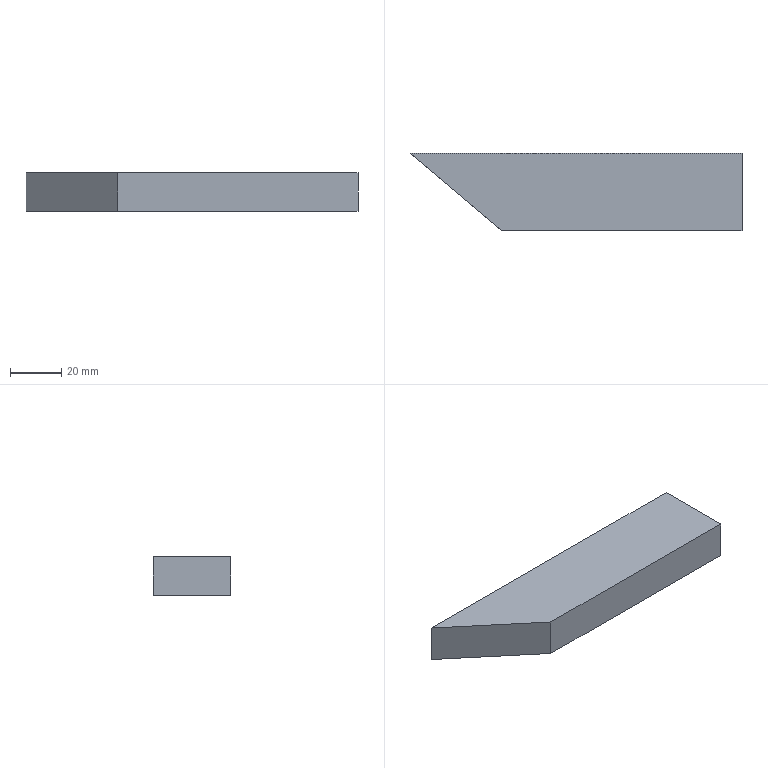Part | NX | features solid 2 | 1 solid | 6 faces | box 129.171 x 30 x 15 mm | volume 50083 mm3 | plane 6
STEP:
#1=CARTESIAN_POINT('',(-96.794,70.,-30.));
#2=VERTEX_POINT('',#1);
#3=CARTESIAN_POINT('',(-61.041,40.,-30.));
#4=VERTEX_POINT('',#3);
#5=CARTESIAN_POINT('',(-95.209,68.67,-30.));
#6=DIRECTION('',(0.766,-0.6428,0.));
#7=VECTOR('',#6,1000.);
#8=LINE('',#5,#7);
#9=EDGE_CURVE('',#2,#4,#8,.T.);
#10=ORIENTED_EDGE('',*,*,#9,.T.);
#11=CARTESIAN_POINT('',(-61.041,40.,-15.));
#12=VERTEX_POINT('',#11);
#13=CARTESIAN_POINT('',(-61.041,40.,-30.));
#14=DIRECTION('',(0.,0.,1.));
#15=VECTOR('',#14,1000.);
#16=LINE('',#13,#15);
#17=EDGE_CURVE('',#4,#12,#16,.T.);
#18=ORIENTED_EDGE('',*,*,#17,.T.);
#19=CARTESIAN_POINT('',(-96.794,70.,-15.));
#20=VERTEX_POINT('',#19);
#21=CARTESIAN_POINT('',(-62.071,40.864,-15.));
#22=DIRECTION('',(-0.766,0.6428,0.));
#23=VECTOR('',#22,1000.);
#24=LINE('',#21,#23);
#25=EDGE_CURVE('',#20,#12,#24,.F.);
#26=ORIENTED_EDGE('',*,*,#25,.F.);
#27=CARTESIAN_POINT('',(-96.794,70.,-30.));
#28=DIRECTION('',(0.,0.,1.));
#29=VECTOR('',#28,1000.);
#30=LINE('',#27,#29);
#31=EDGE_CURVE('',#2,#20,#30,.T.);
#32=ORIENTED_EDGE('',*,*,#31,.F.);
#33=EDGE_LOOP('',(#10,#18,#26,#32));
#34=FACE_BOUND('',#33,.T.);
#35=CARTESIAN_POINT('',(-95.209,68.67,-30.));
#36=DIRECTION('',(0.6428,0.766,0.));
#37=DIRECTION('',(-0.766,0.6428,0.));
#38=AXIS2_PLACEMENT_3D('',#35,#36,#37);
#39=PLANE('',#38);
#40=ADVANCED_FACE('',(#34),#39,.F.);
#41=ORIENTED_EDGE('',*,*,#25,.T.);
#42=CARTESIAN_POINT('',(32.377,40.,-15.));
#43=VERTEX_POINT('',#42);
#44=CARTESIAN_POINT('',(-37.623,40.,-15.));
#45=DIRECTION('',(1.,0.,0.));
#46=VECTOR('',#45,1000.);
#47=LINE('',#44,#46);
#48=EDGE_CURVE('',#12,#43,#47,.T.);
#49=ORIENTED_EDGE('',*,*,#48,.T.);
#50=CARTESIAN_POINT('',(32.377,70.,-15.));
#51=VERTEX_POINT('',#50);
#52=CARTESIAN_POINT('',(32.377,70.,-15.));
#53=DIRECTION('',(0.,1.,0.));
#54=VECTOR('',#53,1000.);
#55=LINE('',#52,#54);
#56=EDGE_CURVE('',#51,#43,#55,.F.);
#57=ORIENTED_EDGE('',*,*,#56,.F.);
#58=CARTESIAN_POINT('',(-37.623,70.,-15.));
#59=DIRECTION('',(1.,0.,0.));
#60=VECTOR('',#59,1000.);
#61=LINE('',#58,#60);
#62=EDGE_CURVE('',#20,#51,#61,.T.);
#63=ORIENTED_EDGE('',*,*,#62,.F.);
#64=EDGE_LOOP('',(#41,#49,#57,#63));
#65=FACE_BOUND('',#64,.T.);
#66=CARTESIAN_POINT('',(-37.623,70.,-15.));
#67=DIRECTION('',(0.,0.,1.));
#68=DIRECTION('',(1.,0.,0.));
#69=AXIS2_PLACEMENT_3D('',#66,#67,#68);
#70=PLANE('',#69);
#71=ADVANCED_FACE('',(#65),#70,.T.);
#72=ORIENTED_EDGE('',*,*,#56,.T.);
#73=CARTESIAN_POINT('',(32.377,40.,-30.));
#74=VERTEX_POINT('',#73);
#75=CARTESIAN_POINT('',(32.377,40.,-30.));
#76=DIRECTION('',(0.,0.,1.));
#77=VECTOR('',#76,1000.);
#78=LINE('',#75,#77);
#79=EDGE_CURVE('',#74,#43,#78,.T.);
#80=ORIENTED_EDGE('',*,*,#79,.F.);
#81=CARTESIAN_POINT('',(32.377,70.,-30.));
#82=VERTEX_POINT('',#81);
#83=CARTESIAN_POINT('',(32.377,70.,-30.));
#84=DIRECTION('',(0.,-1.,0.));
#85=VECTOR('',#84,1000.);
#86=LINE('',#83,#85);
#87=EDGE_CURVE('',#82,#74,#86,.T.);
#88=ORIENTED_EDGE('',*,*,#87,.F.);
#89=CARTESIAN_POINT('',(32.377,70.,-30.));
#90=DIRECTION('',(0.,0.,1.));
#91=VECTOR('',#90,1000.);
#92=LINE('',#89,#91);
#93=EDGE_CURVE('',#82,#51,#92,.T.);
#94=ORIENTED_EDGE('',*,*,#93,.T.);
#95=EDGE_LOOP('',(#72,#80,#88,#94));
#96=FACE_BOUND('',#95,.T.);
#97=CARTESIAN_POINT('',(32.377,70.,-30.));
#98=DIRECTION('',(-1.,0.,0.));
#99=DIRECTION('',(0.,0.,1.));
#100=AXIS2_PLACEMENT_3D('',#97,#98,#99);
#101=PLANE('',#100);
#102=ADVANCED_FACE('',(#96),#101,.F.);
#103=CARTESIAN_POINT('',(-37.623,70.,-30.));
#104=DIRECTION('',(1.,0.,0.));
#105=VECTOR('',#104,1000.);
#106=LINE('',#103,#105);
#107=EDGE_CURVE('',#2,#82,#106,.T.);
#108=ORIENTED_EDGE('',*,*,#107,.T.);
#109=ORIENTED_EDGE('',*,*,#87,.T.);
#110=CARTESIAN_POINT('',(-37.623,40.,-30.));
#111=DIRECTION('',(1.,0.,0.));
#112=VECTOR('',#111,1000.);
#113=LINE('',#110,#112);
#114=EDGE_CURVE('',#4,#74,#113,.T.);
#115=ORIENTED_EDGE('',*,*,#114,.F.);
#116=ORIENTED_EDGE('',*,*,#9,.F.);
#117=EDGE_LOOP('',(#108,#109,#115,#116));
#118=FACE_BOUND('',#117,.T.);
#119=CARTESIAN_POINT('',(-37.623,70.,-30.));
#120=DIRECTION('',(0.,0.,1.));
#121=DIRECTION('',(1.,0.,0.));
#122=AXIS2_PLACEMENT_3D('',#119,#120,#121);
#123=PLANE('',#122);
#124=ADVANCED_FACE('',(#118),#123,.F.);
#125=ORIENTED_EDGE('',*,*,#79,.T.);
#126=ORIENTED_EDGE('',*,*,#48,.F.);
#127=ORIENTED_EDGE('',*,*,#17,.F.);
#128=ORIENTED_EDGE('',*,*,#114,.T.);
#129=EDGE_LOOP('',(#125,#126,#127,#128));
#130=FACE_BOUND('',#129,.T.);
#131=CARTESIAN_POINT('',(-37.623,40.,-30.));
#132=DIRECTION('',(0.,1.,0.));
#133=DIRECTION('',(0.,0.,1.));
#134=AXIS2_PLACEMENT_3D('',#131,#132,#133);
#135=PLANE('',#134);
#136=ADVANCED_FACE('',(#130),#135,.F.);
#137=ORIENTED_EDGE('',*,*,#93,.F.);
#138=ORIENTED_EDGE('',*,*,#107,.F.);
#139=ORIENTED_EDGE('',*,*,#31,.T.);
#140=ORIENTED_EDGE('',*,*,#62,.T.);
#141=EDGE_LOOP('',(#137,#138,#139,#140));
#142=FACE_BOUND('',#141,.T.);
#143=CARTESIAN_POINT('',(-37.623,70.,-30.));
#144=DIRECTION('',(0.,1.,0.));
#145=DIRECTION('',(0.,0.,1.));
#146=AXIS2_PLACEMENT_3D('',#143,#144,#145);
#147=PLANE('',#146);
#148=ADVANCED_FACE('',(#142),#147,.T.);
#149=CLOSED_SHELL('',(#40,#71,#102,#124,#136,#148));
#150=MANIFOLD_SOLID_BREP('',#149);
#151=(LENGTH_UNIT()NAMED_UNIT(*)SI_UNIT(.MILLI.,.METRE.));
#152=UNCERTAINTY_MEASURE_WITH_UNIT(LENGTH_MEASURE(0.00001),#151,'','');
#153=(NAMED_UNIT(*)PLANE_ANGLE_UNIT()SI_UNIT($,.RADIAN.));
#154=(NAMED_UNIT(*)SI_UNIT($,.STERADIAN.)SOLID_ANGLE_UNIT());
#155=(GEOMETRIC_REPRESENTATION_CONTEXT(3)GLOBAL_UNCERTAINTY_ASSIGNED_CONTEXT((#152))GLOBAL_UNIT_ASSIGNED_CONTEXT((#151,#153,#154))REPRESENTATION_CONTEXT('',''));
#156=ADVANCED_BREP_SHAPE_REPRESENTATION('',(#150),#155);